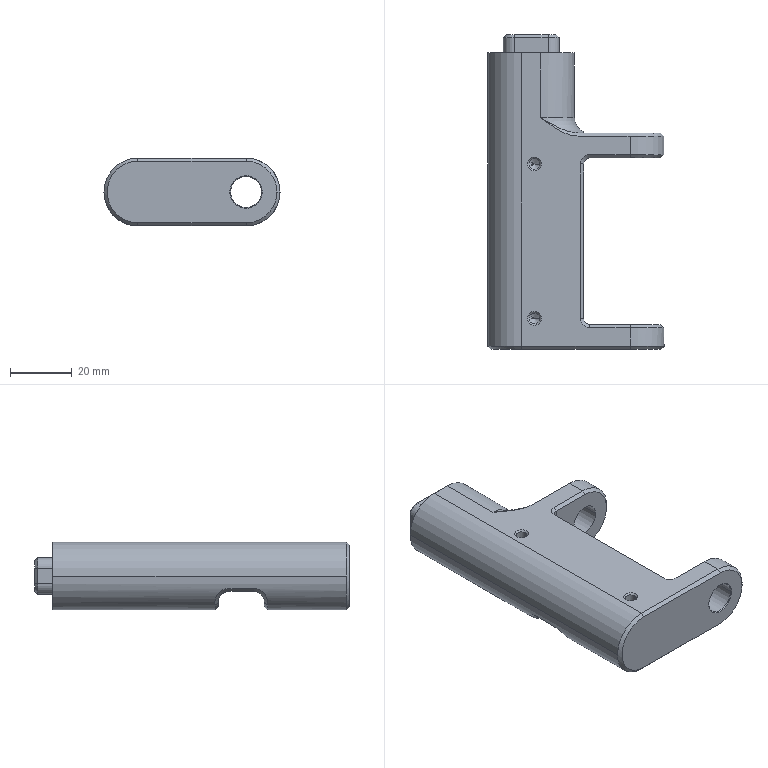Part | SolidWorks | features BaseBody 1 | 1 solid | 114 faces | box 57 x 101.9 x 22 mm | volume 62102 mm3 | plane 41 | cone 40 | cylinder 27 | spline 4 | torus 2 | commonest cylinder face diameters 7 x6 22 x5 3.5 x4 4.8 x4 10 x4 4 x2